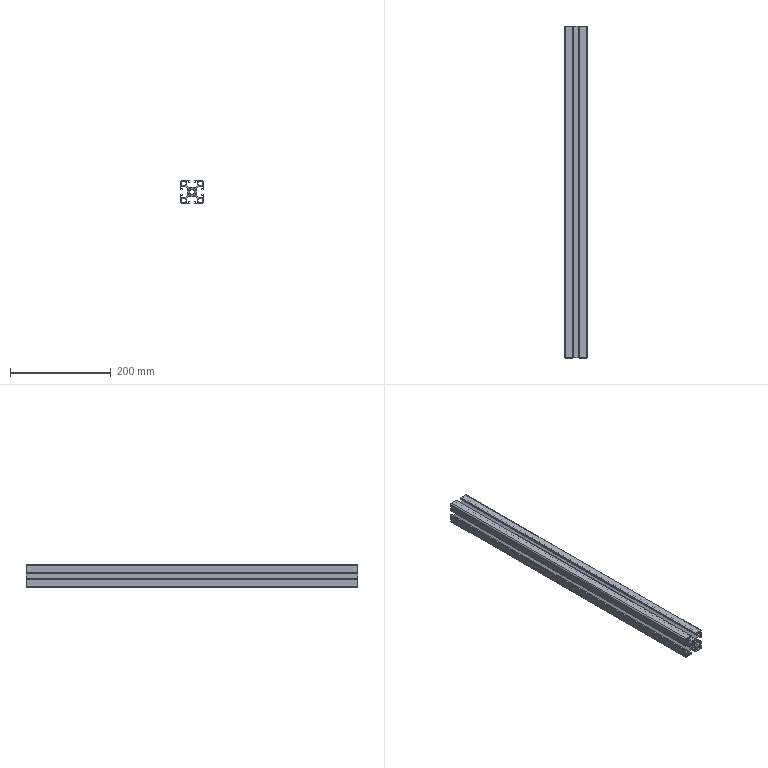Part | STEP file | 1 solid | 135 faces | box 45 x 658 x 45 mm | volume 455527 mm3 | plane 118 | cylinder 17 | commonest cylinder face diameters 10 x9 3 x4 5 x4